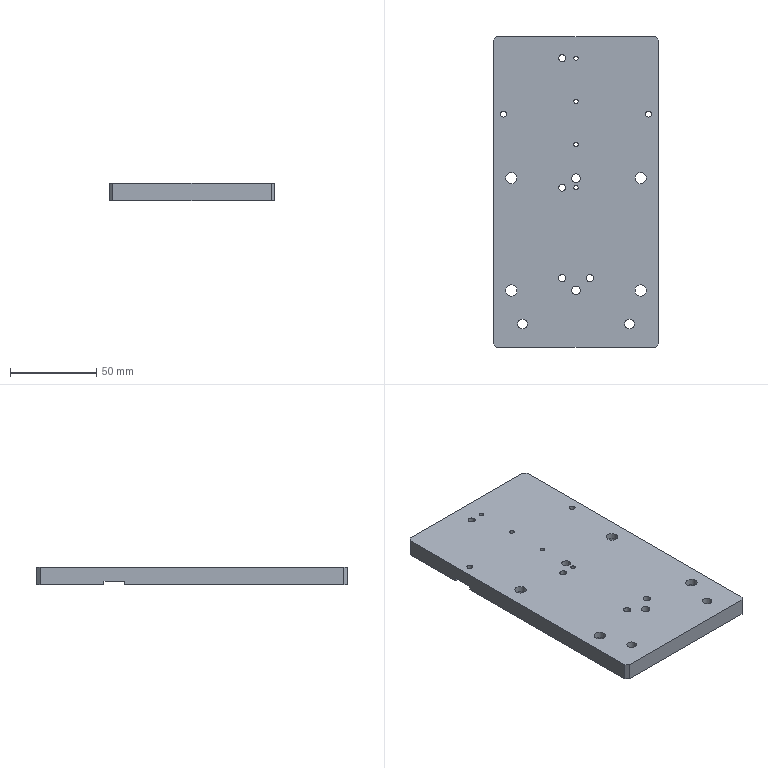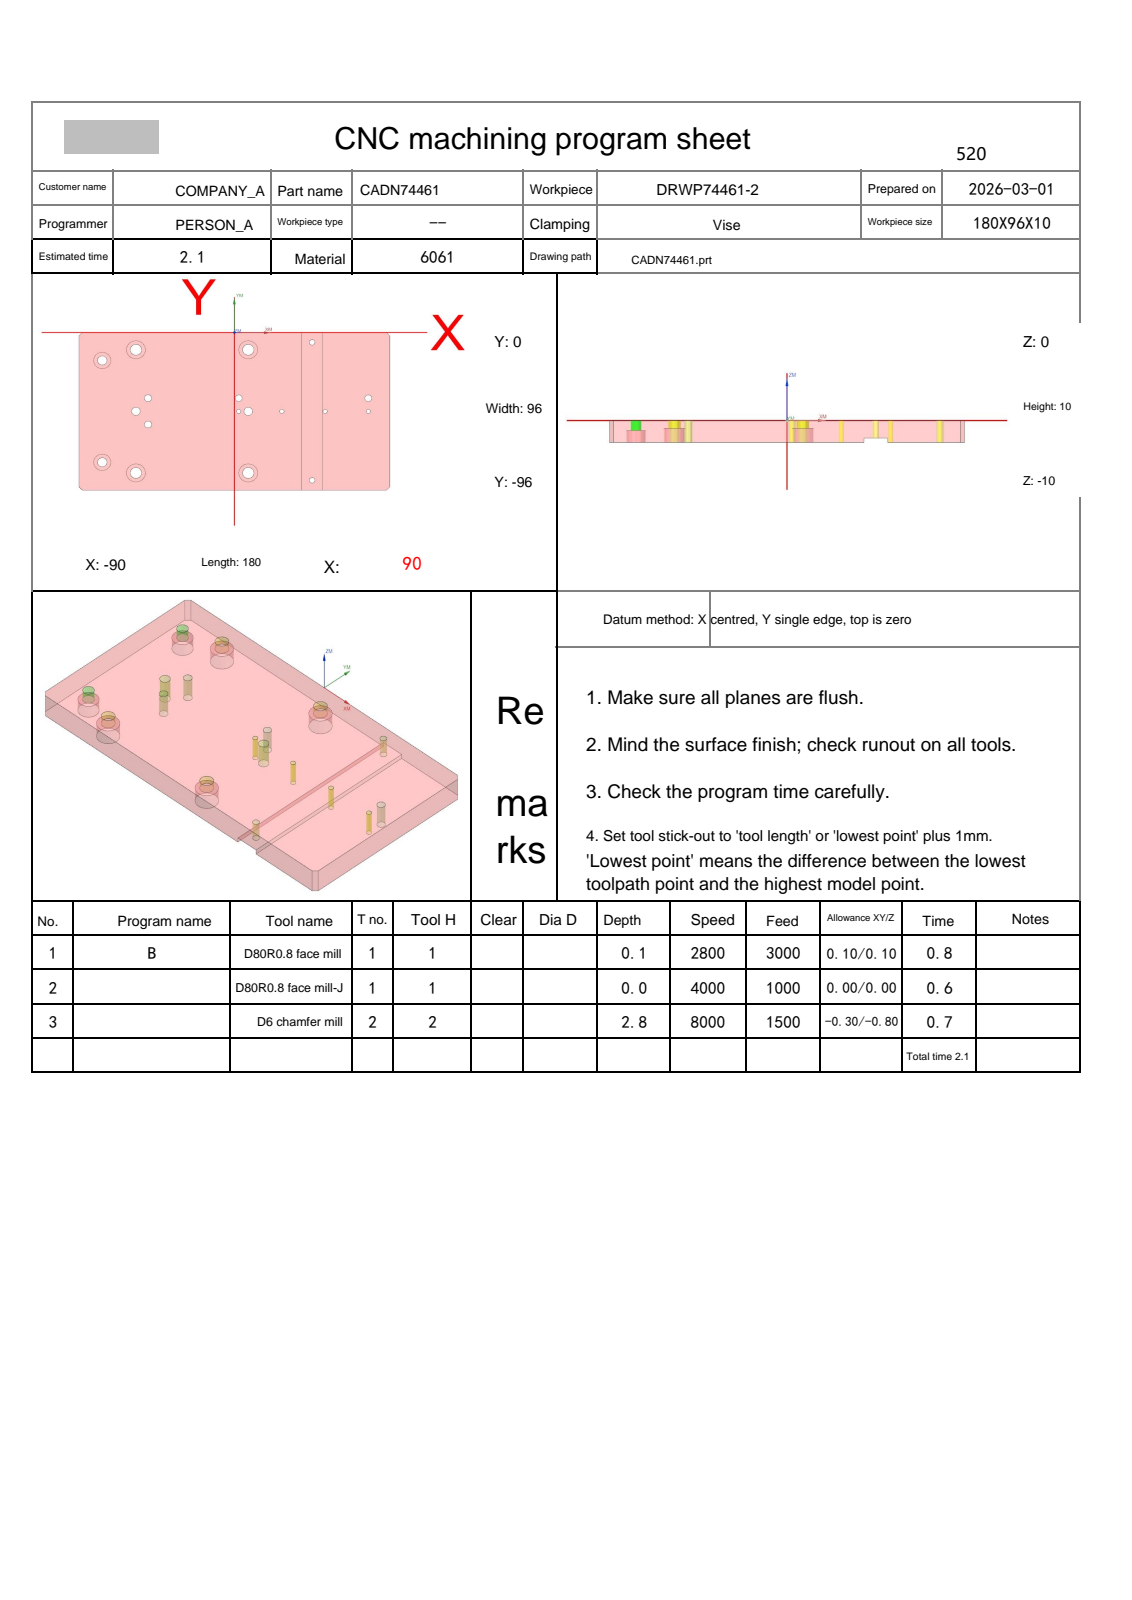NC program | NX | posted by the shop | part box 96 x 180 x 10 mm
Whole program:
%
O0001
(Machine time: 2.69 MIN)
(===Total Tool:2===)
(T1=D80R0.8 face mill D=80.  R=0.8  D-  H01 Z=-0.   )
(T2=D6 chamfer mill   D=6.   R=0.   D-  H02 Z=-2.8  )
G80 G90 G17 G49 G40
G91 G28 Z0
M01
N1 T01 M06
(D80R0.8 face mill  D=80. R=0.8 H=01 ce=0.10 di=0.10)
G00 G90 G54 X-142.097 Y-23.903 M03 S2800
G43 H01 Z50.
M08
Z3.525
G01 Z1.525 F3000.
X-130.097
X122.897
G02 X130.097 Y-31.103 I0.0 J-7.2
G01 Y-56.737
G02 X122.097 Y-64.737 I-8. J0.0
G01 X-130.097
X-142.097
Z3.525
G00 Y-23.903
Z3.05
G01 Z1.05
X-130.097
X122.897
G02 X130.097 Y-31.103 I0.0 J-7.2
G01 Y-56.737
G02 X122.097 Y-64.737 I-8. J0.0
G01 X-130.097
X-142.097
Z3.05
G00 Y-23.903
Z2.575
G01 Z.575
X-130.097
X122.897
G02 X130.097 Y-31.103 I0.0 J-7.2
G01 Y-56.737
G02 X122.097 Y-64.737 I-8. J0.0
G01 X-130.097
X-142.097
Z2.575
G00 Y-23.903
Z2.1
G01 Z.1
X-130.097
X122.897
G02 X130.097 Y-31.103 I0.0 J-7.2
G01 Y-56.737
G02 X122.097 Y-64.737 I-8. J0.0
G01 X-130.097
X-142.097
Z2.1
G00 Z50.
G91 G28 Z0.0
M05
M09
G91 G28 Z0.0
M01
N2 T01 M06
(D80R0.8 face mill-J  D=80. R=0.8 H=01 ce=0.00 di=0.00)
G00 G90 G54 X-141.999 Y-24.001 M03 S4000
G43 H01 Z50.
M08
Z2.
G01 Z0.0 F1000.
X-129.999
X122.799
G02 X129.999 Y-31.201 I0.0 J-7.2
G01 Y-56.639
G02 X121.999 Y-64.639 I-8. J0.0
G01 X-129.999
X-141.999
Z2.
G00 Z50.
G91 G28 Z0.0
M05
M09
G91 G28 Z0.0
M01
N3 T02 M06
(D6 chamfer mill  D=6. R=0. H=02 ce=0.00 di=0.00)
G00 G90 G54 X2.5 Y-48. M03 S8000
G43 H02 Z50.
M08
G98 G81 X2.5 Y-48. Z-1.75 R3. F1000.
X27.5
X52.5
X77.5
G80
G00 Z50.
G00 G90 X45. Y-90. M03 S8000
Z50.
G98 G81 X45. Y-90. Z-2.2 R3. F1000.
Y-6.
G80
G00 Z50.
G00 G90 X77.5 Y-40. M03 S8000
Z50.
G98 G81 X77.5 Y-40. Z-2.3 R3. F1000.
X2.5
G80
G00 Z50.
G00 G90 X8. Y-48. M03 S8000
Z50.
G98 G81 X8. Y-48. Z-2.8 R3. F1000.
X-57.
G80
G00 Z50.
G00 G90 X-50. Y-40. M03 S8000
Z50.
G98 G81 X-50. Y-40. Z-2.7 R3. F1000.
Y-56.
G80
G00 Z50.
G00 G90 X-77.147 Y-17.065 M03 S8000
Z50.
Z-.9
G01 Z-1.4 F1200.
X-78. Y-17.15
G03 X-76.5 Y-18.65 I1.5 J0.0
X-74.85 Y-17. I0.0 J1.65
X-76.5 Y-15.35 I-1.65 J0.0
X-78.15 Y-17. I0.0 J-1.65
X-76.5 Y-18.65 I1.65 J0.0
X-75. Y-17.15 I0.0 J1.5
G01 X-75.853 Y-17.065
Z-.9
G00 Z50.
X-77.147 Y-79.065
Z-.9
G01 Z-1.4
X-78. Y-79.15
G03 X-76.5 Y-80.65 I1.5 J0.0
X-74.85 Y-79. I0.0 J1.65
X-76.5 Y-77.35 I-1.65 J0.0
X-78.15 Y-79. I0.0 J-1.65
X-76.5 Y-80.65 I1.65 J0.0
X-75. Y-79.15 I0.0 J1.5
G01 X-75.853 Y-79.065
Z-.9
G00 Z50.
G00 G90 X6.913 Y-86.007 M03 S8000
Z50.
Z-.9
G01 Z-1.4 F1200.
X6.5 Y-86.2
G03 X8. Y-87.7 I1.5 J0.0
X10.2 Y-85.5 I0.0 J2.2
X8. Y-83.3 I-2.2 J0.0
X5.8 Y-85.5 I0.0 J-2.2
X8. Y-87.7 I2.2 J0.0
X9.5 Y-86.2 I0.0 J1.5
G01 X9.087 Y-86.007
Z-.9
G00 Z50.
X-58.087
Z-.9
G01 Z-1.4
X-58.5 Y-86.2
G03 X-57. Y-87.7 I1.5 J0.0
X-54.8 Y-85.5 I0.0 J2.2
X-57. Y-83.3 I-2.2 J0.0
X-59.2 Y-85.5 I0.0 J-2.2
X-57. Y-87.7 I2.2 J0.0
X-55.5 Y-86.2 I0.0 J1.5
G01 X-55.913 Y-86.007
Z-.9
G00 Z50.
X-58.087 Y-11.007
Z-.9
G01 Z-1.4
X-58.5 Y-11.2
G03 X-57. Y-12.7 I1.5 J0.0
X-54.8 Y-10.5 I0.0 J2.2
X-57. Y-8.3 I-2.2 J0.0
X-59.2 Y-10.5 I0.0 J-2.2
X-57. Y-12.7 I2.2 J0.0
X-55.5 Y-11.2 I0.0 J1.5
G01 X-55.913 Y-11.007
Z-.9
G00 Z50.
X6.913
Z-.9
G01 Z-1.4
X6.5 Y-11.2
G03 X8. Y-12.7 I1.5 J0.0
X10.2 Y-10.5 I0.0 J2.2
X8. Y-8.3 I-2.2 J0.0
X5.8 Y-10.5 I0.0 J-2.2
X8. Y-12.7 I2.2 J0.0
X9.5 Y-11.2 I0.0 J1.5
G01 X9.087 Y-11.007
Z-.9
G00 Z50.
G00 G90 X-79.046 Y-96.7 M03 S7000
Z50.
Z2.5
G01 X-87.953 Z-.742 F1500.
X-88.16 Y-96.662 Z-.819
X-88.355 Y-96.581 Z-.895
X-88.528 Y-96.462 Z-.972
X-88.583 Y-96.407 Z-1.
X-90.407 Y-94.583
G02 X-90.7 Y-93.876 I.707 J.707
G01 Y-2.124
G02 X-90.407 Y-1.417 I1. J0.0
G01 X-88.583 Y.407
G02 X-87.876 Y.7 I.707 J-.707
G01 X87.876
G02 X88.583 Y.407 I0.0 J-1.
G01 X90.407 Y-1.417
G02 X90.7 Y-2.124 I-.707 J-.707
G01 Y-93.876
G02 X90.407 Y-94.583 I-1. J0.0
G01 X88.583 Y-96.407
G02 X87.876 Y-96.7 I-.707 J.707
G01 X-87.876
G02 X-88.583 Y-96.407 I0.0 J1.
G01 X-88.936 Y-96.054
Z1.5
G00 Z50.
M05
M09
G91 G28 Z0.0
G91 G28 Y0.0
M30
%